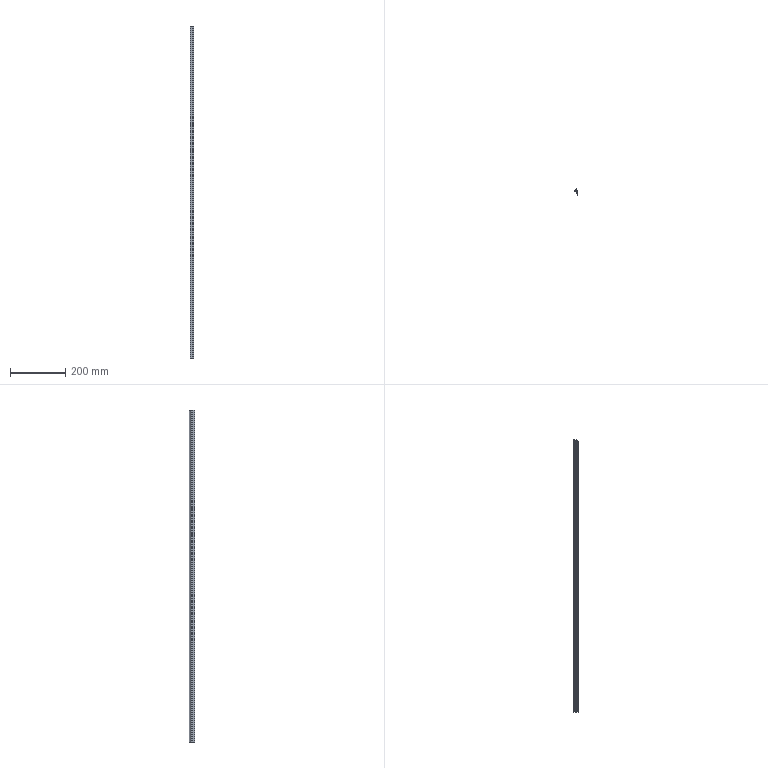Part | SolidWorks | features BaseBody 1, ICE 1, MoveFace 1 | 1 solid | 27 faces | box 14 x 20.3 x 1197 mm | volume 60946 mm3 | plane 20 | cylinder 7 | commonest cylinder face diameters 0.387 x2 0.8 x2 0.4 x1 20 x1 22 x1
STEP:
#1=CARTESIAN_POINT('',(-5.304,-0.625,200.));
#2=VERTEX_POINT('',#1);
#3=CARTESIAN_POINT('',(-5.449,-0.8125,200.));
#4=VERTEX_POINT('',#3);
#5=CARTESIAN_POINT('',(-5.255,-0.8125,200.));
#6=DIRECTION('',(0.,0.,1.));
#7=DIRECTION('',(-1.,0.,0.));
#8=AXIS2_PLACEMENT_3D('',#5,#6,#7);
#9=CIRCLE('',#8,0.1937);
#10=EDGE_CURVE('',#2,#4,#9,.T.);
#11=ORIENTED_EDGE('',*,*,#10,.T.);
#12=CARTESIAN_POINT('',(-5.449,-0.8125,-997.));
#13=VERTEX_POINT('',#12);
#14=CARTESIAN_POINT('',(-5.449,-0.8125,230.));
#15=DIRECTION('',(0.,0.,-1.));
#16=VECTOR('',#15,1000.);
#17=LINE('',#14,#16);
#18=EDGE_CURVE('',#4,#13,#17,.T.);
#19=ORIENTED_EDGE('',*,*,#18,.T.);
#20=CARTESIAN_POINT('',(-5.304,-0.625,-997.));
#21=VERTEX_POINT('',#20);
#22=CARTESIAN_POINT('',(-5.255,-0.8125,-997.));
#23=DIRECTION('',(0.,0.,-1.));
#24=DIRECTION('',(1.,0.,0.));
#25=AXIS2_PLACEMENT_3D('',#22,#23,#24);
#26=CIRCLE('',#25,0.1937);
#27=EDGE_CURVE('',#13,#21,#26,.T.);
#28=ORIENTED_EDGE('',*,*,#27,.T.);
#29=CARTESIAN_POINT('',(-5.304,-0.625,230.));
#30=DIRECTION('',(0.,0.,-1.));
#31=VECTOR('',#30,1000.);
#32=LINE('',#29,#31);
#33=EDGE_CURVE('',#2,#21,#32,.T.);
#34=ORIENTED_EDGE('',*,*,#33,.F.);
#35=EDGE_LOOP('',(#11,#19,#28,#34));
#36=FACE_OUTER_BOUND('',#35,.T.);
#37=CARTESIAN_POINT('',(-5.255,-0.8125,230.));
#38=DIRECTION('',(0.,0.,-1.));
#39=DIRECTION('',(-1.,0.,0.));
#40=AXIS2_PLACEMENT_3D('',#37,#38,#39);
#41=CYLINDRICAL_SURFACE('',#40,0.1937);
#42=ADVANCED_FACE('',(#36),#41,.F.);
#43=CARTESIAN_POINT('',(5.,-1.,-997.));
#44=VERTEX_POINT('',#43);
#45=CARTESIAN_POINT('',(5.,-14.3,-997.));
#46=VERTEX_POINT('',#45);
#47=CARTESIAN_POINT('',(5.,29.623,-997.));
#48=DIRECTION('',(0.,-1.,0.));
#49=VECTOR('',#48,1000.);
#50=LINE('',#47,#49);
#51=EDGE_CURVE('',#44,#46,#50,.T.);
#52=ORIENTED_EDGE('',*,*,#51,.F.);
#53=CARTESIAN_POINT('',(5.,-1.,200.));
#54=VERTEX_POINT('',#53);
#55=CARTESIAN_POINT('',(5.,-1.,230.));
#56=DIRECTION('',(0.,0.,-1.));
#57=VECTOR('',#56,1000.);
#58=LINE('',#55,#57);
#59=EDGE_CURVE('',#54,#44,#58,.T.);
#60=ORIENTED_EDGE('',*,*,#59,.F.);
#61=CARTESIAN_POINT('',(5.,-14.3,200.));
#62=VERTEX_POINT('',#61);
#63=CARTESIAN_POINT('',(5.,-14.3,200.));
#64=DIRECTION('',(0.,1.,0.));
#65=VECTOR('',#64,1000.);
#66=LINE('',#63,#65);
#67=EDGE_CURVE('',#62,#54,#66,.T.);
#68=ORIENTED_EDGE('',*,*,#67,.F.);
#69=CARTESIAN_POINT('',(5.,-14.3,230.));
#70=DIRECTION('',(0.,0.,1.));
#71=VECTOR('',#70,1000.);
#72=LINE('',#69,#71);
#73=EDGE_CURVE('',#46,#62,#72,.T.);
#74=ORIENTED_EDGE('',*,*,#73,.F.);
#75=EDGE_LOOP('',(#52,#60,#68,#74));
#76=FACE_OUTER_BOUND('',#75,.T.);
#77=CARTESIAN_POINT('',(5.,-14.3,230.));
#78=DIRECTION('',(-1.,0.,0.));
#79=DIRECTION('',(0.,0.,1.));
#80=AXIS2_PLACEMENT_3D('',#77,#78,#79);
#81=PLANE('',#80);
#82=ADVANCED_FACE('',(#76),#81,.F.);
#83=CARTESIAN_POINT('',(-9.,-2.,-997.));
#84=VERTEX_POINT('',#83);
#85=CARTESIAN_POINT('',(-9.,-2.,200.));
#86=VERTEX_POINT('',#85);
#87=CARTESIAN_POINT('',(-9.,-2.,230.));
#88=DIRECTION('',(0.,0.,1.));
#89=VECTOR('',#88,1000.);
#90=LINE('',#87,#89);
#91=EDGE_CURVE('',#84,#86,#90,.T.);
#92=ORIENTED_EDGE('',*,*,#91,.F.);
#93=CARTESIAN_POINT('',(0.9,-2.,-997.));
#94=VERTEX_POINT('',#93);
#95=CARTESIAN_POINT('',(5.,-2.,-997.));
#96=DIRECTION('',(-1.,0.,0.));
#97=VECTOR('',#96,1000.);
#98=LINE('',#95,#97);
#99=EDGE_CURVE('',#94,#84,#98,.T.);
#100=ORIENTED_EDGE('',*,*,#99,.F.);
#101=CARTESIAN_POINT('',(0.9,-2.,200.));
#102=VERTEX_POINT('',#101);
#103=CARTESIAN_POINT('',(0.9,-2.,230.));
#104=DIRECTION('',(0.,0.,-1.));
#105=VECTOR('',#104,1000.);
#106=LINE('',#103,#105);
#107=EDGE_CURVE('',#102,#94,#106,.T.);
#108=ORIENTED_EDGE('',*,*,#107,.F.);
#109=CARTESIAN_POINT('',(5.,-2.,200.));
#110=DIRECTION('',(1.,0.,0.));
#111=VECTOR('',#110,1000.);
#112=LINE('',#109,#111);
#113=EDGE_CURVE('',#86,#102,#112,.T.);
#114=ORIENTED_EDGE('',*,*,#113,.F.);
#115=EDGE_LOOP('',(#92,#100,#108,#114));
#116=FACE_OUTER_BOUND('',#115,.T.);
#117=CARTESIAN_POINT('',(-9.,-2.,230.));
#118=DIRECTION('',(0.,1.,0.));
#119=DIRECTION('',(0.,0.,1.));
#120=AXIS2_PLACEMENT_3D('',#117,#118,#119);
#121=PLANE('',#120);
#122=ADVANCED_FACE('',(#116),#121,.F.);
#123=CARTESIAN_POINT('',(4.,-6.,200.));
#124=VERTEX_POINT('',#123);
#125=CARTESIAN_POINT('',(4.,-3.,200.));
#126=VERTEX_POINT('',#125);
#127=CARTESIAN_POINT('',(4.,29.623,200.));
#128=DIRECTION('',(0.,1.,0.));
#129=VECTOR('',#128,1000.);
#130=LINE('',#127,#129);
#131=EDGE_CURVE('',#124,#126,#130,.T.);
#132=ORIENTED_EDGE('',*,*,#131,.F.);
#133=CARTESIAN_POINT('',(1.,-6.,200.));
#134=VERTEX_POINT('',#133);
#135=CARTESIAN_POINT('',(5.,-6.,200.));
#136=DIRECTION('',(1.,0.,0.));
#137=VECTOR('',#136,1000.);
#138=LINE('',#135,#137);
#139=EDGE_CURVE('',#134,#124,#138,.T.);
#140=ORIENTED_EDGE('',*,*,#139,.F.);
#141=CARTESIAN_POINT('',(1.,-6.7,200.));
#142=VERTEX_POINT('',#141);
#143=CARTESIAN_POINT('',(1.,-6.,200.));
#144=DIRECTION('',(0.,-1.,0.));
#145=VECTOR('',#144,1000.);
#146=LINE('',#143,#145);
#147=EDGE_CURVE('',#134,#142,#146,.T.);
#148=ORIENTED_EDGE('',*,*,#147,.T.);
#149=CARTESIAN_POINT('',(-1.7,-6.7,200.));
#150=VERTEX_POINT('',#149);
#151=CARTESIAN_POINT('',(5.,-6.7,200.));
#152=DIRECTION('',(1.,0.,0.));
#153=VECTOR('',#152,1000.);
#154=LINE('',#151,#153);
#155=EDGE_CURVE('',#150,#142,#154,.T.);
#156=ORIENTED_EDGE('',*,*,#155,.F.);
#157=CARTESIAN_POINT('',(-1.7,-7.7,200.));
#158=VERTEX_POINT('',#157);
#159=CARTESIAN_POINT('',(-1.7,-6.7,200.));
#160=DIRECTION('',(0.,-1.,0.));
#161=VECTOR('',#160,1000.);
#162=LINE('',#159,#161);
#163=EDGE_CURVE('',#150,#158,#162,.T.);
#164=ORIENTED_EDGE('',*,*,#163,.T.);
#165=CARTESIAN_POINT('',(4.,-7.7,200.));
#166=VERTEX_POINT('',#165);
#167=CARTESIAN_POINT('',(5.,-7.7,200.));
#168=DIRECTION('',(-1.,0.,0.));
#169=VECTOR('',#168,1000.);
#170=LINE('',#167,#169);
#171=EDGE_CURVE('',#166,#158,#170,.T.);
#172=ORIENTED_EDGE('',*,*,#171,.F.);
#173=CARTESIAN_POINT('',(4.,-14.3,200.));
#174=VERTEX_POINT('',#173);
#175=CARTESIAN_POINT('',(4.,29.623,200.));
#176=DIRECTION('',(0.,1.,0.));
#177=VECTOR('',#176,1000.);
#178=LINE('',#175,#177);
#179=EDGE_CURVE('',#174,#166,#178,.T.);
#180=ORIENTED_EDGE('',*,*,#179,.F.);
#181=CARTESIAN_POINT('',(5.,-14.3,200.));
#182=DIRECTION('',(-1.,0.,0.));
#183=VECTOR('',#182,1000.);
#184=LINE('',#181,#183);
#185=EDGE_CURVE('',#62,#174,#184,.T.);
#186=ORIENTED_EDGE('',*,*,#185,.F.);
#187=ORIENTED_EDGE('',*,*,#67,.T.);
#188=CARTESIAN_POINT('',(-5.207,-1.,200.));
#189=VERTEX_POINT('',#188);
#190=CARTESIAN_POINT('',(5.,-1.,200.));
#191=DIRECTION('',(1.,0.,0.));
#192=VECTOR('',#191,1000.);
#193=LINE('',#190,#192);
#194=EDGE_CURVE('',#189,#54,#193,.T.);
#195=ORIENTED_EDGE('',*,*,#194,.F.);
#196=CARTESIAN_POINT('',(-5.255,-0.8125,200.));
#197=DIRECTION('',(0.,0.,1.));
#198=DIRECTION('',(-1.,0.,0.));
#199=AXIS2_PLACEMENT_3D('',#196,#197,#198);
#200=CIRCLE('',#199,0.1937);
#201=EDGE_CURVE('',#4,#189,#200,.T.);
#202=ORIENTED_EDGE('',*,*,#201,.F.);
#203=ORIENTED_EDGE('',*,*,#10,.F.);
#204=CARTESIAN_POINT('',(-1.368,3.063,200.));
#205=VERTEX_POINT('',#204);
#206=CARTESIAN_POINT('',(-10.628,9.,200.));
#207=DIRECTION('',(0.,0.,1.));
#208=DIRECTION('',(-1.,0.,0.));
#209=AXIS2_PLACEMENT_3D('',#206,#207,#208);
#210=CIRCLE('',#209,11.);
#211=EDGE_CURVE('',#2,#205,#210,.T.);
#212=ORIENTED_EDGE('',*,*,#211,.T.);
#213=CARTESIAN_POINT('',(-1.,2.955,200.));
#214=VERTEX_POINT('',#213);
#215=CARTESIAN_POINT('',(-1.2,2.955,200.));
#216=DIRECTION('',(0.,0.,1.));
#217=DIRECTION('',(-1.,0.,0.));
#218=AXIS2_PLACEMENT_3D('',#215,#216,#217);
#219=CIRCLE('',#218,0.2);
#220=EDGE_CURVE('',#214,#205,#219,.T.);
#221=ORIENTED_EDGE('',*,*,#220,.F.);
#222=CARTESIAN_POINT('',(-1.,1.5,200.));
#223=VERTEX_POINT('',#222);
#224=CARTESIAN_POINT('',(-1.,2.955,200.));
#225=DIRECTION('',(0.,1.,0.));
#226=VECTOR('',#225,1000.);
#227=LINE('',#224,#226);
#228=EDGE_CURVE('',#223,#214,#227,.T.);
#229=ORIENTED_EDGE('',*,*,#228,.F.);
#230=CARTESIAN_POINT('',(0.,1.5,200.));
#231=VERTEX_POINT('',#230);
#232=CARTESIAN_POINT('',(-1.,1.5,200.));
#233=DIRECTION('',(-1.,0.,0.));
#234=VECTOR('',#233,1000.);
#235=LINE('',#232,#234);
#236=EDGE_CURVE('',#231,#223,#235,.T.);
#237=ORIENTED_EDGE('',*,*,#236,.F.);
#238=CARTESIAN_POINT('',(0.,6.,200.));
#239=VERTEX_POINT('',#238);
#240=CARTESIAN_POINT('',(0.,1.5,200.));
#241=DIRECTION('',(0.,-1.,0.));
#242=VECTOR('',#241,1000.);
#243=LINE('',#240,#242);
#244=EDGE_CURVE('',#239,#231,#243,.T.);
#245=ORIENTED_EDGE('',*,*,#244,.F.);
#246=CARTESIAN_POINT('',(-0.8,6.,200.));
#247=VERTEX_POINT('',#246);
#248=CARTESIAN_POINT('',(0.,6.,200.));
#249=DIRECTION('',(1.,0.,0.));
#250=VECTOR('',#249,1000.);
#251=LINE('',#248,#250);
#252=EDGE_CURVE('',#247,#239,#251,.T.);
#253=ORIENTED_EDGE('',*,*,#252,.F.);
#254=CARTESIAN_POINT('',(-1.178,5.731,200.));
#255=VERTEX_POINT('',#254);
#256=CARTESIAN_POINT('',(-0.8,5.6,200.));
#257=DIRECTION('',(0.,0.,1.));
#258=DIRECTION('',(-1.,0.,0.));
#259=AXIS2_PLACEMENT_3D('',#256,#257,#258);
#260=CIRCLE('',#259,0.4);
#261=EDGE_CURVE('',#247,#255,#260,.T.);
#262=ORIENTED_EDGE('',*,*,#261,.T.);
#263=CARTESIAN_POINT('',(-8.678,-0.8077,200.));
#264=VERTEX_POINT('',#263);
#265=CARTESIAN_POINT('',(-10.628,9.,200.));
#266=DIRECTION('',(0.,0.,1.));
#267=DIRECTION('',(-1.,0.,0.));
#268=AXIS2_PLACEMENT_3D('',#265,#266,#267);
#269=CIRCLE('',#268,10.);
#270=EDGE_CURVE('',#264,#255,#269,.T.);
#271=ORIENTED_EDGE('',*,*,#270,.F.);
#272=CARTESIAN_POINT('',(-9.,-1.2,200.));
#273=VERTEX_POINT('',#272);
#274=CARTESIAN_POINT('',(-8.6,-1.2,200.));
#275=DIRECTION('',(0.,0.,1.));
#276=DIRECTION('',(-1.,0.,0.));
#277=AXIS2_PLACEMENT_3D('',#274,#275,#276);
#278=CIRCLE('',#277,0.4);
#279=EDGE_CURVE('',#264,#273,#278,.T.);
#280=ORIENTED_EDGE('',*,*,#279,.T.);
#281=CARTESIAN_POINT('',(-9.,8.,200.));
#282=DIRECTION('',(0.,-1.,0.));
#283=VECTOR('',#282,1000.);
#284=LINE('',#281,#283);
#285=EDGE_CURVE('',#273,#86,#284,.T.);
#286=ORIENTED_EDGE('',*,*,#285,.T.);
#287=ORIENTED_EDGE('',*,*,#113,.T.);
#288=CARTESIAN_POINT('',(0.9,-3.,200.));
#289=VERTEX_POINT('',#288);
#290=CARTESIAN_POINT('',(0.9,29.623,200.));
#291=DIRECTION('',(0.,1.,0.));
#292=VECTOR('',#291,1000.);
#293=LINE('',#290,#292);
#294=EDGE_CURVE('',#289,#102,#293,.T.);
#295=ORIENTED_EDGE('',*,*,#294,.F.);
#296=CARTESIAN_POINT('',(5.,-3.,200.));
#297=DIRECTION('',(-1.,0.,0.));
#298=VECTOR('',#297,1000.);
#299=LINE('',#296,#298);
#300=EDGE_CURVE('',#126,#289,#299,.T.);
#301=ORIENTED_EDGE('',*,*,#300,.F.);
#302=EDGE_LOOP('',(#132,#140,#148,#156,#164,#172,#180,#186,#187,#195,#202,#203,#212,#221,#229,#237,#245,#253,#262,#271,#280,#286,#287,#295,#301));
#303=FACE_OUTER_BOUND('',#302,.T.);
#304=CARTESIAN_POINT('',(5.,29.623,200.));
#305=DIRECTION('',(0.,0.,-1.));
#306=DIRECTION('',(-1.,0.,0.));
#307=AXIS2_PLACEMENT_3D('',#304,#305,#306);
#308=PLANE('',#307);
#309=ADVANCED_FACE('',(#303),#308,.F.);
#310=ORIENTED_EDGE('',*,*,#185,.T.);
#311=CARTESIAN_POINT('',(4.,-14.3,-997.));
#312=VERTEX_POINT('',#311);
#313=CARTESIAN_POINT('',(4.,-14.3,230.));
#314=DIRECTION('',(0.,0.,1.));
#315=VECTOR('',#314,1000.);
#316=LINE('',#313,#315);
#317=EDGE_CURVE('',#312,#174,#316,.T.);
#318=ORIENTED_EDGE('',*,*,#317,.F.);
#319=CARTESIAN_POINT('',(5.,-14.3,-997.));
#320=DIRECTION('',(-1.,0.,0.));
#321=VECTOR('',#320,1000.);
#322=LINE('',#319,#321);
#323=EDGE_CURVE('',#46,#312,#322,.T.);
#324=ORIENTED_EDGE('',*,*,#323,.F.);
#325=ORIENTED_EDGE('',*,*,#73,.T.);
#326=EDGE_LOOP('',(#310,#318,#324,#325));
#327=FACE_OUTER_BOUND('',#326,.T.);
#328=CARTESIAN_POINT('',(4.,-14.3,230.));
#329=DIRECTION('',(0.,1.,0.));
#330=DIRECTION('',(0.,0.,1.));
#331=AXIS2_PLACEMENT_3D('',#328,#329,#330);
#332=PLANE('',#331);
#333=ADVANCED_FACE('',(#327),#332,.F.);
#334=ORIENTED_EDGE('',*,*,#51,.T.);
#335=ORIENTED_EDGE('',*,*,#323,.T.);
#336=CARTESIAN_POINT('',(4.,-7.7,-997.));
#337=VERTEX_POINT('',#336);
#338=CARTESIAN_POINT('',(4.,-7.7,-997.));
#339=DIRECTION('',(0.,-1.,0.));
#340=VECTOR('',#339,1000.);
#341=LINE('',#338,#340);
#342=EDGE_CURVE('',#337,#312,#341,.T.);
#343=ORIENTED_EDGE('',*,*,#342,.F.);
#344=CARTESIAN_POINT('',(-1.7,-7.7,-997.));
#345=VERTEX_POINT('',#344);
#346=CARTESIAN_POINT('',(-1.7,-7.7,-997.));
#347=DIRECTION('',(1.,0.,0.));
#348=VECTOR('',#347,1000.);
#349=LINE('',#346,#348);
#350=EDGE_CURVE('',#345,#337,#349,.T.);
#351=ORIENTED_EDGE('',*,*,#350,.F.);
#352=CARTESIAN_POINT('',(-1.7,-6.7,-997.));
#353=VERTEX_POINT('',#352);
#354=CARTESIAN_POINT('',(-1.7,29.623,-997.));
#355=DIRECTION('',(0.,1.,0.));
#356=VECTOR('',#355,1000.);
#357=LINE('',#354,#356);
#358=EDGE_CURVE('',#345,#353,#357,.T.);
#359=ORIENTED_EDGE('',*,*,#358,.T.);
#360=CARTESIAN_POINT('',(1.,-6.7,-997.));
#361=VERTEX_POINT('',#360);
#362=CARTESIAN_POINT('',(1.,-6.7,-997.));
#363=DIRECTION('',(-1.,0.,0.));
#364=VECTOR('',#363,1000.);
#365=LINE('',#362,#364);
#366=EDGE_CURVE('',#361,#353,#365,.T.);
#367=ORIENTED_EDGE('',*,*,#366,.F.);
#368=CARTESIAN_POINT('',(1.,-6.,-997.));
#369=VERTEX_POINT('',#368);
#370=CARTESIAN_POINT('',(1.,29.623,-997.));
#371=DIRECTION('',(0.,1.,0.));
#372=VECTOR('',#371,1000.);
#373=LINE('',#370,#372);
#374=EDGE_CURVE('',#361,#369,#373,.T.);
#375=ORIENTED_EDGE('',*,*,#374,.T.);
#376=CARTESIAN_POINT('',(4.,-6.,-997.));
#377=VERTEX_POINT('',#376);
#378=CARTESIAN_POINT('',(4.,-6.,-997.));
#379=DIRECTION('',(-1.,0.,0.));
#380=VECTOR('',#379,1000.);
#381=LINE('',#378,#380);
#382=EDGE_CURVE('',#377,#369,#381,.T.);
#383=ORIENTED_EDGE('',*,*,#382,.F.);
#384=CARTESIAN_POINT('',(4.,-3.,-997.));
#385=VERTEX_POINT('',#384);
#386=CARTESIAN_POINT('',(4.,-3.,-997.));
#387=DIRECTION('',(0.,-1.,0.));
#388=VECTOR('',#387,1000.);
#389=LINE('',#386,#388);
#390=EDGE_CURVE('',#385,#377,#389,.T.);
#391=ORIENTED_EDGE('',*,*,#390,.F.);
#392=CARTESIAN_POINT('',(0.9,-3.,-997.));
#393=VERTEX_POINT('',#392);
#394=CARTESIAN_POINT('',(0.9,-3.,-997.));
#395=DIRECTION('',(1.,0.,0.));
#396=VECTOR('',#395,1000.);
#397=LINE('',#394,#396);
#398=EDGE_CURVE('',#393,#385,#397,.T.);
#399=ORIENTED_EDGE('',*,*,#398,.F.);
#400=CARTESIAN_POINT('',(0.9,-2.,-997.));
#401=DIRECTION('',(0.,-1.,0.));
#402=VECTOR('',#401,1000.);
#403=LINE('',#400,#402);
#404=EDGE_CURVE('',#94,#393,#403,.T.);
#405=ORIENTED_EDGE('',*,*,#404,.F.);
#406=ORIENTED_EDGE('',*,*,#99,.T.);
#407=CARTESIAN_POINT('',(-9.,-1.2,-997.));
#408=VERTEX_POINT('',#407);
#409=CARTESIAN_POINT('',(-9.,-1.2,-997.));
#410=DIRECTION('',(0.,-1.,0.));
#411=VECTOR('',#410,1000.);
#412=LINE('',#409,#411);
#413=EDGE_CURVE('',#408,#84,#412,.T.);
#414=ORIENTED_EDGE('',*,*,#413,.F.);
#415=CARTESIAN_POINT('',(-8.678,-0.8077,-997.));
#416=VERTEX_POINT('',#415);
#417=CARTESIAN_POINT('',(-8.6,-1.2,-997.));
#418=DIRECTION('',(0.,0.,-1.));
#419=DIRECTION('',(1.,0.,0.));
#420=AXIS2_PLACEMENT_3D('',#417,#418,#419);
#421=CIRCLE('',#420,0.4);
#422=EDGE_CURVE('',#408,#416,#421,.T.);
#423=ORIENTED_EDGE('',*,*,#422,.T.);
#424=CARTESIAN_POINT('',(-1.178,5.731,-997.));
#425=VERTEX_POINT('',#424);
#426=CARTESIAN_POINT('',(-10.628,9.,-997.));
#427=DIRECTION('',(0.,0.,-1.));
#428=DIRECTION('',(1.,0.,0.));
#429=AXIS2_PLACEMENT_3D('',#426,#427,#428);
#430=CIRCLE('',#429,10.);
#431=EDGE_CURVE('',#425,#416,#430,.T.);
#432=ORIENTED_EDGE('',*,*,#431,.F.);
#433=CARTESIAN_POINT('',(-0.8,6.,-997.));
#434=VERTEX_POINT('',#433);
#435=CARTESIAN_POINT('',(-0.8,5.6,-997.));
#436=DIRECTION('',(0.,0.,-1.));
#437=DIRECTION('',(1.,0.,0.));
#438=AXIS2_PLACEMENT_3D('',#435,#436,#437);
#439=CIRCLE('',#438,0.4);
#440=EDGE_CURVE('',#425,#434,#439,.T.);
#441=ORIENTED_EDGE('',*,*,#440,.T.);
#442=CARTESIAN_POINT('',(0.,6.,-997.));
#443=VERTEX_POINT('',#442);
#444=CARTESIAN_POINT('',(0.,6.,-997.));
#445=DIRECTION('',(-1.,0.,0.));
#446=VECTOR('',#445,1000.);
#447=LINE('',#444,#446);
#448=EDGE_CURVE('',#443,#434,#447,.T.);
#449=ORIENTED_EDGE('',*,*,#448,.F.);
#450=CARTESIAN_POINT('',(0.,1.5,-997.));
#451=VERTEX_POINT('',#450);
#452=CARTESIAN_POINT('',(0.,1.5,-997.));
#453=DIRECTION('',(0.,1.,0.));
#454=VECTOR('',#453,1000.);
#455=LINE('',#452,#454);
#456=EDGE_CURVE('',#451,#443,#455,.T.);
#457=ORIENTED_EDGE('',*,*,#456,.F.);
#458=CARTESIAN_POINT('',(-1.,1.5,-997.));
#459=VERTEX_POINT('',#458);
#460=CARTESIAN_POINT('',(-1.,1.5,-997.));
#461=DIRECTION('',(1.,0.,0.));
#462=VECTOR('',#461,1000.);
#463=LINE('',#460,#462);
#464=EDGE_CURVE('',#459,#451,#463,.T.);
#465=ORIENTED_EDGE('',*,*,#464,.F.);
#466=CARTESIAN_POINT('',(-1.,2.955,-997.));
#467=VERTEX_POINT('',#466);
#468=CARTESIAN_POINT('',(-1.,2.955,-997.));
#469=DIRECTION('',(0.,-1.,0.));
#470=VECTOR('',#469,1000.);
#471=LINE('',#468,#470);
#472=EDGE_CURVE('',#467,#459,#471,.T.);
#473=ORIENTED_EDGE('',*,*,#472,.F.);
#474=CARTESIAN_POINT('',(-1.368,3.063,-997.));
#475=VERTEX_POINT('',#474);
#476=CARTESIAN_POINT('',(-1.2,2.955,-997.));
#477=DIRECTION('',(0.,0.,-1.));
#478=DIRECTION('',(1.,0.,0.));
#479=AXIS2_PLACEMENT_3D('',#476,#477,#478);
#480=CIRCLE('',#479,0.2);
#481=EDGE_CURVE('',#475,#467,#480,.T.);
#482=ORIENTED_EDGE('',*,*,#481,.F.);
#483=CARTESIAN_POINT('',(-10.628,9.,-997.));
#484=DIRECTION('',(0.,0.,-1.));
#485=DIRECTION('',(1.,0.,0.));
#486=AXIS2_PLACEMENT_3D('',#483,#484,#485);
#487=CIRCLE('',#486,11.);
#488=EDGE_CURVE('',#475,#21,#487,.T.);
#489=ORIENTED_EDGE('',*,*,#488,.T.);
#490=ORIENTED_EDGE('',*,*,#27,.F.);
#491=CARTESIAN_POINT('',(-5.207,-1.,-997.));
#492=VERTEX_POINT('',#491);
#493=CARTESIAN_POINT('',(-5.255,-0.8125,-997.));
#494=DIRECTION('',(0.,0.,-1.));
#495=DIRECTION('',(1.,0.,0.));
#496=AXIS2_PLACEMENT_3D('',#493,#494,#495);
#497=CIRCLE('',#496,0.1937);
#498=EDGE_CURVE('',#492,#13,#497,.T.);
#499=ORIENTED_EDGE('',*,*,#498,.F.);
#500=CARTESIAN_POINT('',(5.,-1.,-997.));
#501=DIRECTION('',(-1.,0.,0.));
#502=VECTOR('',#501,1000.);
#503=LINE('',#500,#502);
#504=EDGE_CURVE('',#44,#492,#503,.T.);
#505=ORIENTED_EDGE('',*,*,#504,.F.);
#506=EDGE_LOOP('',(#334,#335,#343,#351,#359,#367,#375,#383,#391,#399,#405,#406,#414,#423,#432,#441,#449,#457,#465,#473,#482,#489,#490,#499,#505));
#507=FACE_OUTER_BOUND('',#506,.T.);
#508=CARTESIAN_POINT('',(5.,29.623,-997.));
#509=DIRECTION('',(0.,0.,1.));
#510=DIRECTION('',(1.,0.,0.));
#511=AXIS2_PLACEMENT_3D('',#508,#509,#510);
#512=PLANE('',#511);
#513=ADVANCED_FACE('',(#507),#512,.F.);
#514=ORIENTED_EDGE('',*,*,#59,.T.);
#515=ORIENTED_EDGE('',*,*,#504,.T.);
#516=CARTESIAN_POINT('',(-5.207,-1.,230.));
#517=DIRECTION('',(0.,0.,-1.));
#518=VECTOR('',#517,1000.);
#519=LINE('',#516,#518);
#520=EDGE_CURVE('',#189,#492,#519,.T.);
#521=ORIENTED_EDGE('',*,*,#520,.F.);
#522=ORIENTED_EDGE('',*,*,#194,.T.);
#523=EDGE_LOOP('',(#514,#515,#521,#522));
#524=FACE_OUTER_BOUND('',#523,.T.);
#525=CARTESIAN_POINT('',(5.,-1.,230.));
#526=DIRECTION('',(0.,-1.,0.));
#527=DIRECTION('',(0.,0.,-1.));
#528=AXIS2_PLACEMENT_3D('',#525,#526,#527);
#529=PLANE('',#528);
#530=ADVANCED_FACE('',(#524),#529,.F.);
#531=CARTESIAN_POINT('',(-9.,-1.2,230.));
#532=DIRECTION('',(0.,0.,1.));
#533=VECTOR('',#532,1000.);
#534=LINE('',#531,#533);
#535=EDGE_CURVE('',#408,#273,#534,.T.);
#536=ORIENTED_EDGE('',*,*,#535,.F.);
#537=ORIENTED_EDGE('',*,*,#413,.T.);
#538=ORIENTED_EDGE('',*,*,#91,.T.);
#539=ORIENTED_EDGE('',*,*,#285,.F.);
#540=EDGE_LOOP('',(#536,#537,#538,#539));
#541=FACE_OUTER_BOUND('',#540,.T.);
#542=CARTESIAN_POINT('',(-9.,-1.2,230.));
#543=DIRECTION('',(1.,0.,0.));
#544=DIRECTION('',(0.,0.,-1.));
#545=AXIS2_PLACEMENT_3D('',#542,#543,#544);
#546=PLANE('',#545);
#547=ADVANCED_FACE('',(#541),#546,.F.);
#548=ORIENTED_EDGE('',*,*,#294,.T.);
#549=ORIENTED_EDGE('',*,*,#107,.T.);
#550=ORIENTED_EDGE('',*,*,#404,.T.);
#551=CARTESIAN_POINT('',(0.9,-3.,230.));
#552=DIRECTION('',(0.,0.,-1.));
#553=VECTOR('',#552,1000.);
#554=LINE('',#551,#553);
#555=EDGE_CURVE('',#289,#393,#554,.T.);
#556=ORIENTED_EDGE('',*,*,#555,.F.);
#557=EDGE_LOOP('',(#548,#549,#550,#556));
#558=FACE_OUTER_BOUND('',#557,.T.);
#559=CARTESIAN_POINT('',(0.9,-2.,230.));
#560=DIRECTION('',(1.,0.,0.));
#561=DIRECTION('',(0.,0.,-1.));
#562=AXIS2_PLACEMENT_3D('',#559,#560,#561);
#563=PLANE('',#562);
#564=ADVANCED_FACE('',(#558),#563,.F.);
#565=ORIENTED_EDGE('',*,*,#300,.T.);
#566=ORIENTED_EDGE('',*,*,#555,.T.);
#567=ORIENTED_EDGE('',*,*,#398,.T.);
#568=CARTESIAN_POINT('',(4.,-3.,230.));
#569=DIRECTION('',(0.,0.,-1.));
#570=VECTOR('',#569,1000.);
#571=LINE('',#568,#570);
#572=EDGE_CURVE('',#126,#385,#571,.T.);
#573=ORIENTED_EDGE('',*,*,#572,.F.);
#574=EDGE_LOOP('',(#565,#566,#567,#573));
#575=FACE_OUTER_BOUND('',#574,.T.);
#576=CARTESIAN_POINT('',(0.9,-3.,230.));
#577=DIRECTION('',(0.,1.,0.));
#578=DIRECTION('',(0.,0.,1.));
#579=AXIS2_PLACEMENT_3D('',#576,#577,#578);
#580=PLANE('',#579);
#581=ADVANCED_FACE('',(#575),#580,.F.);
#582=ORIENTED_EDGE('',*,*,#131,.T.);
#583=ORIENTED_EDGE('',*,*,#572,.T.);
#584=ORIENTED_EDGE('',*,*,#390,.T.);
#585=CARTESIAN_POINT('',(4.,-6.,230.));
#586=DIRECTION('',(0.,0.,-1.));
#587=VECTOR('',#586,1000.);
#588=LINE('',#585,#587);
#589=EDGE_CURVE('',#124,#377,#588,.T.);
#590=ORIENTED_EDGE('',*,*,#589,.F.);
#591=EDGE_LOOP('',(#582,#583,#584,#590));
#592=FACE_OUTER_BOUND('',#591,.T.);
#593=CARTESIAN_POINT('',(4.,-3.,230.));
#594=DIRECTION('',(1.,0.,0.));
#595=DIRECTION('',(0.,0.,-1.));
#596=AXIS2_PLACEMENT_3D('',#593,#594,#595);
#597=PLANE('',#596);
#598=ADVANCED_FACE('',(#592),#597,.F.);
#599=ORIENTED_EDGE('',*,*,#139,.T.);
#600=ORIENTED_EDGE('',*,*,#589,.T.);
#601=ORIENTED_EDGE('',*,*,#382,.T.);
#602=CARTESIAN_POINT('',(1.,-6.,230.));
#603=DIRECTION('',(0.,0.,-1.));
#604=VECTOR('',#603,1000.);
#605=LINE('',#602,#604);
#606=EDGE_CURVE('',#134,#369,#605,.T.);
#607=ORIENTED_EDGE('',*,*,#606,.F.);
#608=EDGE_LOOP('',(#599,#600,#601,#607));
#609=FACE_OUTER_BOUND('',#608,.T.);
#610=CARTESIAN_POINT('',(4.,-6.,230.));
#611=DIRECTION('',(0.,-1.,0.));
#612=DIRECTION('',(0.,0.,-1.));
#613=AXIS2_PLACEMENT_3D('',#610,#611,#612);
#614=PLANE('',#613);
#615=ADVANCED_FACE('',(#609),#614,.F.);
#616=ORIENTED_EDGE('',*,*,#155,.T.);
#617=CARTESIAN_POINT('',(1.,-6.7,230.));
#618=DIRECTION('',(0.,0.,1.));
#619=VECTOR('',#618,1000.);
#620=LINE('',#617,#619);
#621=EDGE_CURVE('',#361,#142,#620,.T.);
#622=ORIENTED_EDGE('',*,*,#621,.F.);
#623=ORIENTED_EDGE('',*,*,#366,.T.);
#624=CARTESIAN_POINT('',(-1.7,-6.7,230.));
#625=DIRECTION('',(0.,0.,-1.));
#626=VECTOR('',#625,1000.);
#627=LINE('',#624,#626);
#628=EDGE_CURVE('',#150,#353,#627,.T.);
#629=ORIENTED_EDGE('',*,*,#628,.F.);
#630=EDGE_LOOP('',(#616,#622,#623,#629));
#631=FACE_OUTER_BOUND('',#630,.T.);
#632=CARTESIAN_POINT('',(1.,-6.7,230.));
#633=DIRECTION('',(0.,-1.,0.));
#634=DIRECTION('',(0.,0.,-1.));
#635=AXIS2_PLACEMENT_3D('',#632,#633,#634);
#636=PLANE('',#635);
#637=ADVANCED_FACE('',(#631),#636,.F.);
#638=ORIENTED_EDGE('',*,*,#171,.T.);
#639=CARTESIAN_POINT('',(-1.7,-7.7,230.));
#640=DIRECTION('',(0.,0.,1.));
#641=VECTOR('',#640,1000.);
#642=LINE('',#639,#641);
#643=EDGE_CURVE('',#345,#158,#642,.T.);
#644=ORIENTED_EDGE('',*,*,#643,.F.);
#645=ORIENTED_EDGE('',*,*,#350,.T.);
#646=CARTESIAN_POINT('',(4.,-7.7,230.));
#647=DIRECTION('',(0.,0.,-1.));
#648=VECTOR('',#647,1000.);
#649=LINE('',#646,#648);
#650=EDGE_CURVE('',#166,#337,#649,.T.);
#651=ORIENTED_EDGE('',*,*,#650,.F.);
#652=EDGE_LOOP('',(#638,#644,#645,#651));
#653=FACE_OUTER_BOUND('',#652,.T.);
#654=CARTESIAN_POINT('',(-1.7,-7.7,230.));
#655=DIRECTION('',(0.,1.,0.));
#656=DIRECTION('',(0.,0.,1.));
#657=AXIS2_PLACEMENT_3D('',#654,#655,#656);
#658=PLANE('',#657);
#659=ADVANCED_FACE('',(#653),#658,.F.);
#660=ORIENTED_EDGE('',*,*,#179,.T.);
#661=ORIENTED_EDGE('',*,*,#650,.T.);
#662=ORIENTED_EDGE('',*,*,#342,.T.);
#663=ORIENTED_EDGE('',*,*,#317,.T.);
#664=EDGE_LOOP('',(#660,#661,#662,#663));
#665=FACE_OUTER_BOUND('',#664,.T.);
#666=CARTESIAN_POINT('',(4.,-7.7,230.));
#667=DIRECTION('',(1.,0.,0.));
#668=DIRECTION('',(0.,0.,-1.));
#669=AXIS2_PLACEMENT_3D('',#666,#667,#668);
#670=PLANE('',#669);
#671=ADVANCED_FACE('',(#665),#670,.F.);
#672=ORIENTED_EDGE('',*,*,#18,.F.);
#673=ORIENTED_EDGE('',*,*,#201,.T.);
#674=ORIENTED_EDGE('',*,*,#520,.T.);
#675=ORIENTED_EDGE('',*,*,#498,.T.);
#676=EDGE_LOOP('',(#672,#673,#674,#675));
#677=FACE_OUTER_BOUND('',#676,.T.);
#678=CARTESIAN_POINT('',(-5.255,-0.8125,230.));
#679=DIRECTION('',(0.,0.,-1.));
#680=DIRECTION('',(-1.,0.,0.));
#681=AXIS2_PLACEMENT_3D('',#678,#679,#680);
#682=CYLINDRICAL_SURFACE('',#681,0.1937);
#683=ADVANCED_FACE('',(#677),#682,.F.);
#684=CARTESIAN_POINT('',(-1.,2.955,230.));
#685=DIRECTION('',(0.,0.,1.));
#686=VECTOR('',#685,1000.);
#687=LINE('',#684,#686);
#688=EDGE_CURVE('',#467,#214,#687,.T.);
#689=ORIENTED_EDGE('',*,*,#688,.F.);
#690=ORIENTED_EDGE('',*,*,#472,.T.);
#691=CARTESIAN_POINT('',(-1.,1.5,230.));
#692=DIRECTION('',(0.,0.,-1.));
#693=VECTOR('',#692,1000.);
#694=LINE('',#691,#693);
#695=EDGE_CURVE('',#223,#459,#694,.T.);
#696=ORIENTED_EDGE('',*,*,#695,.F.);
#697=ORIENTED_EDGE('',*,*,#228,.T.);
#698=EDGE_LOOP('',(#689,#690,#696,#697));
#699=FACE_OUTER_BOUND('',#698,.T.);
#700=CARTESIAN_POINT('',(-1.,2.955,230.));
#701=DIRECTION('',(1.,0.,0.));
#702=DIRECTION('',(0.,0.,-1.));
#703=AXIS2_PLACEMENT_3D('',#700,#701,#702);
#704=PLANE('',#703);
#705=ADVANCED_FACE('',(#699),#704,.F.);
#706=ORIENTED_EDGE('',*,*,#488,.F.);
#707=CARTESIAN_POINT('',(-1.368,3.063,230.));
#708=DIRECTION('',(0.,0.,1.));
#709=VECTOR('',#708,1000.);
#710=LINE('',#707,#709);
#711=EDGE_CURVE('',#475,#205,#710,.T.);
#712=ORIENTED_EDGE('',*,*,#711,.T.);
#713=ORIENTED_EDGE('',*,*,#211,.F.);
#714=ORIENTED_EDGE('',*,*,#33,.T.);
#715=EDGE_LOOP('',(#706,#712,#713,#714));
#716=FACE_OUTER_BOUND('',#715,.T.);
#717=CARTESIAN_POINT('',(-10.628,9.,230.));
#718=DIRECTION('',(0.,0.,-1.));
#719=DIRECTION('',(-1.,0.,0.));
#720=AXIS2_PLACEMENT_3D('',#717,#718,#719);
#721=CYLINDRICAL_SURFACE('',#720,11.);
#722=ADVANCED_FACE('',(#716),#721,.T.);
#723=CARTESIAN_POINT('',(-1.178,5.731,230.));
#724=DIRECTION('',(0.,0.,1.));
#725=VECTOR('',#724,1000.);
#726=LINE('',#723,#725);
#727=EDGE_CURVE('',#425,#255,#726,.T.);
#728=ORIENTED_EDGE('',*,*,#727,.F.);
#729=ORIENTED_EDGE('',*,*,#431,.T.);
#730=CARTESIAN_POINT('',(-8.678,-0.8077,230.));
#731=DIRECTION('',(0.,0.,-1.));
#732=VECTOR('',#731,1000.);
#733=LINE('',#730,#732);
#734=EDGE_CURVE('',#264,#416,#733,.T.);
#735=ORIENTED_EDGE('',*,*,#734,.F.);
#736=ORIENTED_EDGE('',*,*,#270,.T.);
#737=EDGE_LOOP('',(#728,#729,#735,#736));
#738=FACE_OUTER_BOUND('',#737,.T.);
#739=CARTESIAN_POINT('',(-10.628,9.,230.));
#740=DIRECTION('',(0.,0.,-1.));
#741=DIRECTION('',(-1.,0.,0.));
#742=AXIS2_PLACEMENT_3D('',#739,#740,#741);
#743=CYLINDRICAL_SURFACE('',#742,10.);
#744=ADVANCED_FACE('',(#738),#743,.F.);
#745=CARTESIAN_POINT('',(0.,1.5,230.));
#746=DIRECTION('',(0.,0.,1.));
#747=VECTOR('',#746,1000.);
#748=LINE('',#745,#747);
#749=EDGE_CURVE('',#451,#231,#748,.T.);
#750=ORIENTED_EDGE('',*,*,#749,.F.);
#751=ORIENTED_EDGE('',*,*,#456,.T.);
#752=CARTESIAN_POINT('',(0.,6.,230.));
#753=DIRECTION('',(0.,0.,-1.));
#754=VECTOR('',#753,1000.);
#755=LINE('',#752,#754);
#756=EDGE_CURVE('',#239,#443,#755,.T.);
#757=ORIENTED_EDGE('',*,*,#756,.F.);
#758=ORIENTED_EDGE('',*,*,#244,.T.);
#759=EDGE_LOOP('',(#750,#751,#757,#758));
#760=FACE_OUTER_BOUND('',#759,.T.);
#761=CARTESIAN_POINT('',(0.,1.5,230.));
#762=DIRECTION('',(-1.,0.,0.));
#763=DIRECTION('',(0.,0.,1.));
#764=AXIS2_PLACEMENT_3D('',#761,#762,#763);
#765=PLANE('',#764);
#766=ADVANCED_FACE('',(#760),#765,.F.);
#767=ORIENTED_EDGE('',*,*,#422,.F.);
#768=ORIENTED_EDGE('',*,*,#535,.T.);
#769=ORIENTED_EDGE('',*,*,#279,.F.);
#770=ORIENTED_EDGE('',*,*,#734,.T.);
#771=EDGE_LOOP('',(#767,#768,#769,#770));
#772=FACE_OUTER_BOUND('',#771,.T.);
#773=CARTESIAN_POINT('',(-8.6,-1.2,230.));
#774=DIRECTION('',(0.,0.,-1.));
#775=DIRECTION('',(-1.,0.,0.));
#776=AXIS2_PLACEMENT_3D('',#773,#774,#775);
#777=CYLINDRICAL_SURFACE('',#776,0.4);
#778=ADVANCED_FACE('',(#772),#777,.T.);
#779=ORIENTED_EDGE('',*,*,#147,.F.);
#780=ORIENTED_EDGE('',*,*,#606,.T.);
#781=ORIENTED_EDGE('',*,*,#374,.F.);
#782=ORIENTED_EDGE('',*,*,#621,.T.);
#783=EDGE_LOOP('',(#779,#780,#781,#782));
#784=FACE_OUTER_BOUND('',#783,.T.);
#785=CARTESIAN_POINT('',(1.,-6.,230.));
#786=DIRECTION('',(1.,0.,0.));
#787=DIRECTION('',(0.,0.,-1.));
#788=AXIS2_PLACEMENT_3D('',#785,#786,#787);
#789=PLANE('',#788);
#790=ADVANCED_FACE('',(#784),#789,.F.);
#791=ORIENTED_EDGE('',*,*,#163,.F.);
#792=ORIENTED_EDGE('',*,*,#628,.T.);
#793=ORIENTED_EDGE('',*,*,#358,.F.);
#794=ORIENTED_EDGE('',*,*,#643,.T.);
#795=EDGE_LOOP('',(#791,#792,#793,#794));
#796=FACE_OUTER_BOUND('',#795,.T.);
#797=CARTESIAN_POINT('',(-1.7,-6.7,230.));
#798=DIRECTION('',(1.,0.,0.));
#799=DIRECTION('',(0.,0.,-1.));
#800=AXIS2_PLACEMENT_3D('',#797,#798,#799);
#801=PLANE('',#800);
#802=ADVANCED_FACE('',(#796),#801,.F.);
#803=ORIENTED_EDGE('',*,*,#711,.F.);
#804=ORIENTED_EDGE('',*,*,#481,.T.);
#805=ORIENTED_EDGE('',*,*,#688,.T.);
#806=ORIENTED_EDGE('',*,*,#220,.T.);
#807=EDGE_LOOP('',(#803,#804,#805,#806));
#808=FACE_OUTER_BOUND('',#807,.T.);
#809=CARTESIAN_POINT('',(-1.2,2.955,230.));
#810=DIRECTION('',(0.,0.,-1.));
#811=DIRECTION('',(-1.,0.,0.));
#812=AXIS2_PLACEMENT_3D('',#809,#810,#811);
#813=CYLINDRICAL_SURFACE('',#812,0.2);
#814=ADVANCED_FACE('',(#808),#813,.F.);
#815=ORIENTED_EDGE('',*,*,#695,.T.);
#816=ORIENTED_EDGE('',*,*,#464,.T.);
#817=ORIENTED_EDGE('',*,*,#749,.T.);
#818=ORIENTED_EDGE('',*,*,#236,.T.);
#819=EDGE_LOOP('',(#815,#816,#817,#818));
#820=FACE_OUTER_BOUND('',#819,.T.);
#821=CARTESIAN_POINT('',(-1.,1.5,230.));
#822=DIRECTION('',(0.,1.,0.));
#823=DIRECTION('',(0.,0.,1.));
#824=AXIS2_PLACEMENT_3D('',#821,#822,#823);
#825=PLANE('',#824);
#826=ADVANCED_FACE('',(#820),#825,.F.);
#827=ORIENTED_EDGE('',*,*,#440,.F.);
#828=ORIENTED_EDGE('',*,*,#727,.T.);
#829=ORIENTED_EDGE('',*,*,#261,.F.);
#830=CARTESIAN_POINT('',(-0.8,6.,230.));
#831=DIRECTION('',(0.,0.,-1.));
#832=VECTOR('',#831,1000.);
#833=LINE('',#830,#832);
#834=EDGE_CURVE('',#247,#434,#833,.T.);
#835=ORIENTED_EDGE('',*,*,#834,.T.);
#836=EDGE_LOOP('',(#827,#828,#829,#835));
#837=FACE_OUTER_BOUND('',#836,.T.);
#838=CARTESIAN_POINT('',(-0.8,5.6,230.));
#839=DIRECTION('',(0.,0.,-1.));
#840=DIRECTION('',(-1.,0.,0.));
#841=AXIS2_PLACEMENT_3D('',#838,#839,#840);
#842=CYLINDRICAL_SURFACE('',#841,0.4);
#843=ADVANCED_FACE('',(#837),#842,.T.);
#844=ORIENTED_EDGE('',*,*,#756,.T.);
#845=ORIENTED_EDGE('',*,*,#448,.T.);
#846=ORIENTED_EDGE('',*,*,#834,.F.);
#847=ORIENTED_EDGE('',*,*,#252,.T.);
#848=EDGE_LOOP('',(#844,#845,#846,#847));
#849=FACE_OUTER_BOUND('',#848,.T.);
#850=CARTESIAN_POINT('',(0.,6.,230.));
#851=DIRECTION('',(0.,-1.,0.));
#852=DIRECTION('',(0.,0.,-1.));
#853=AXIS2_PLACEMENT_3D('',#850,#851,#852);
#854=PLANE('',#853);
#855=ADVANCED_FACE('',(#849),#854,.F.);
#856=CLOSED_SHELL('',(#42,#82,#122,#309,#333,#513,#530,#547,#564,#581,#598,#615,#637,#659,#671,#683,#705,#722,#744,#766,#778,#790,#802,#814,#826,#843,#855));
#857=MANIFOLD_SOLID_BREP('',#856);
#858=CARTESIAN_POINT('',(0.,0.,0.));
#859=DIRECTION('',(0.,0.,1.));
#860=DIRECTION('',(1.,0.,0.));
#861=AXIS2_PLACEMENT_3D('',#858,#859,#860);
#862=(LENGTH_UNIT()NAMED_UNIT(*)SI_UNIT(.MILLI.,.METRE.));
#863=UNCERTAINTY_MEASURE_WITH_UNIT(LENGTH_MEASURE(0.00001),#862,'','');
#864=(NAMED_UNIT(*)PLANE_ANGLE_UNIT()SI_UNIT($,.RADIAN.));
#865=(NAMED_UNIT(*)SI_UNIT($,.STERADIAN.)SOLID_ANGLE_UNIT());
#866=(GEOMETRIC_REPRESENTATION_CONTEXT(3)GLOBAL_UNCERTAINTY_ASSIGNED_CONTEXT((#863))GLOBAL_UNIT_ASSIGNED_CONTEXT((#862,#864,#865))REPRESENTATION_CONTEXT('',''));
#867=ADVANCED_BREP_SHAPE_REPRESENTATION('',(#857,#861),#866);